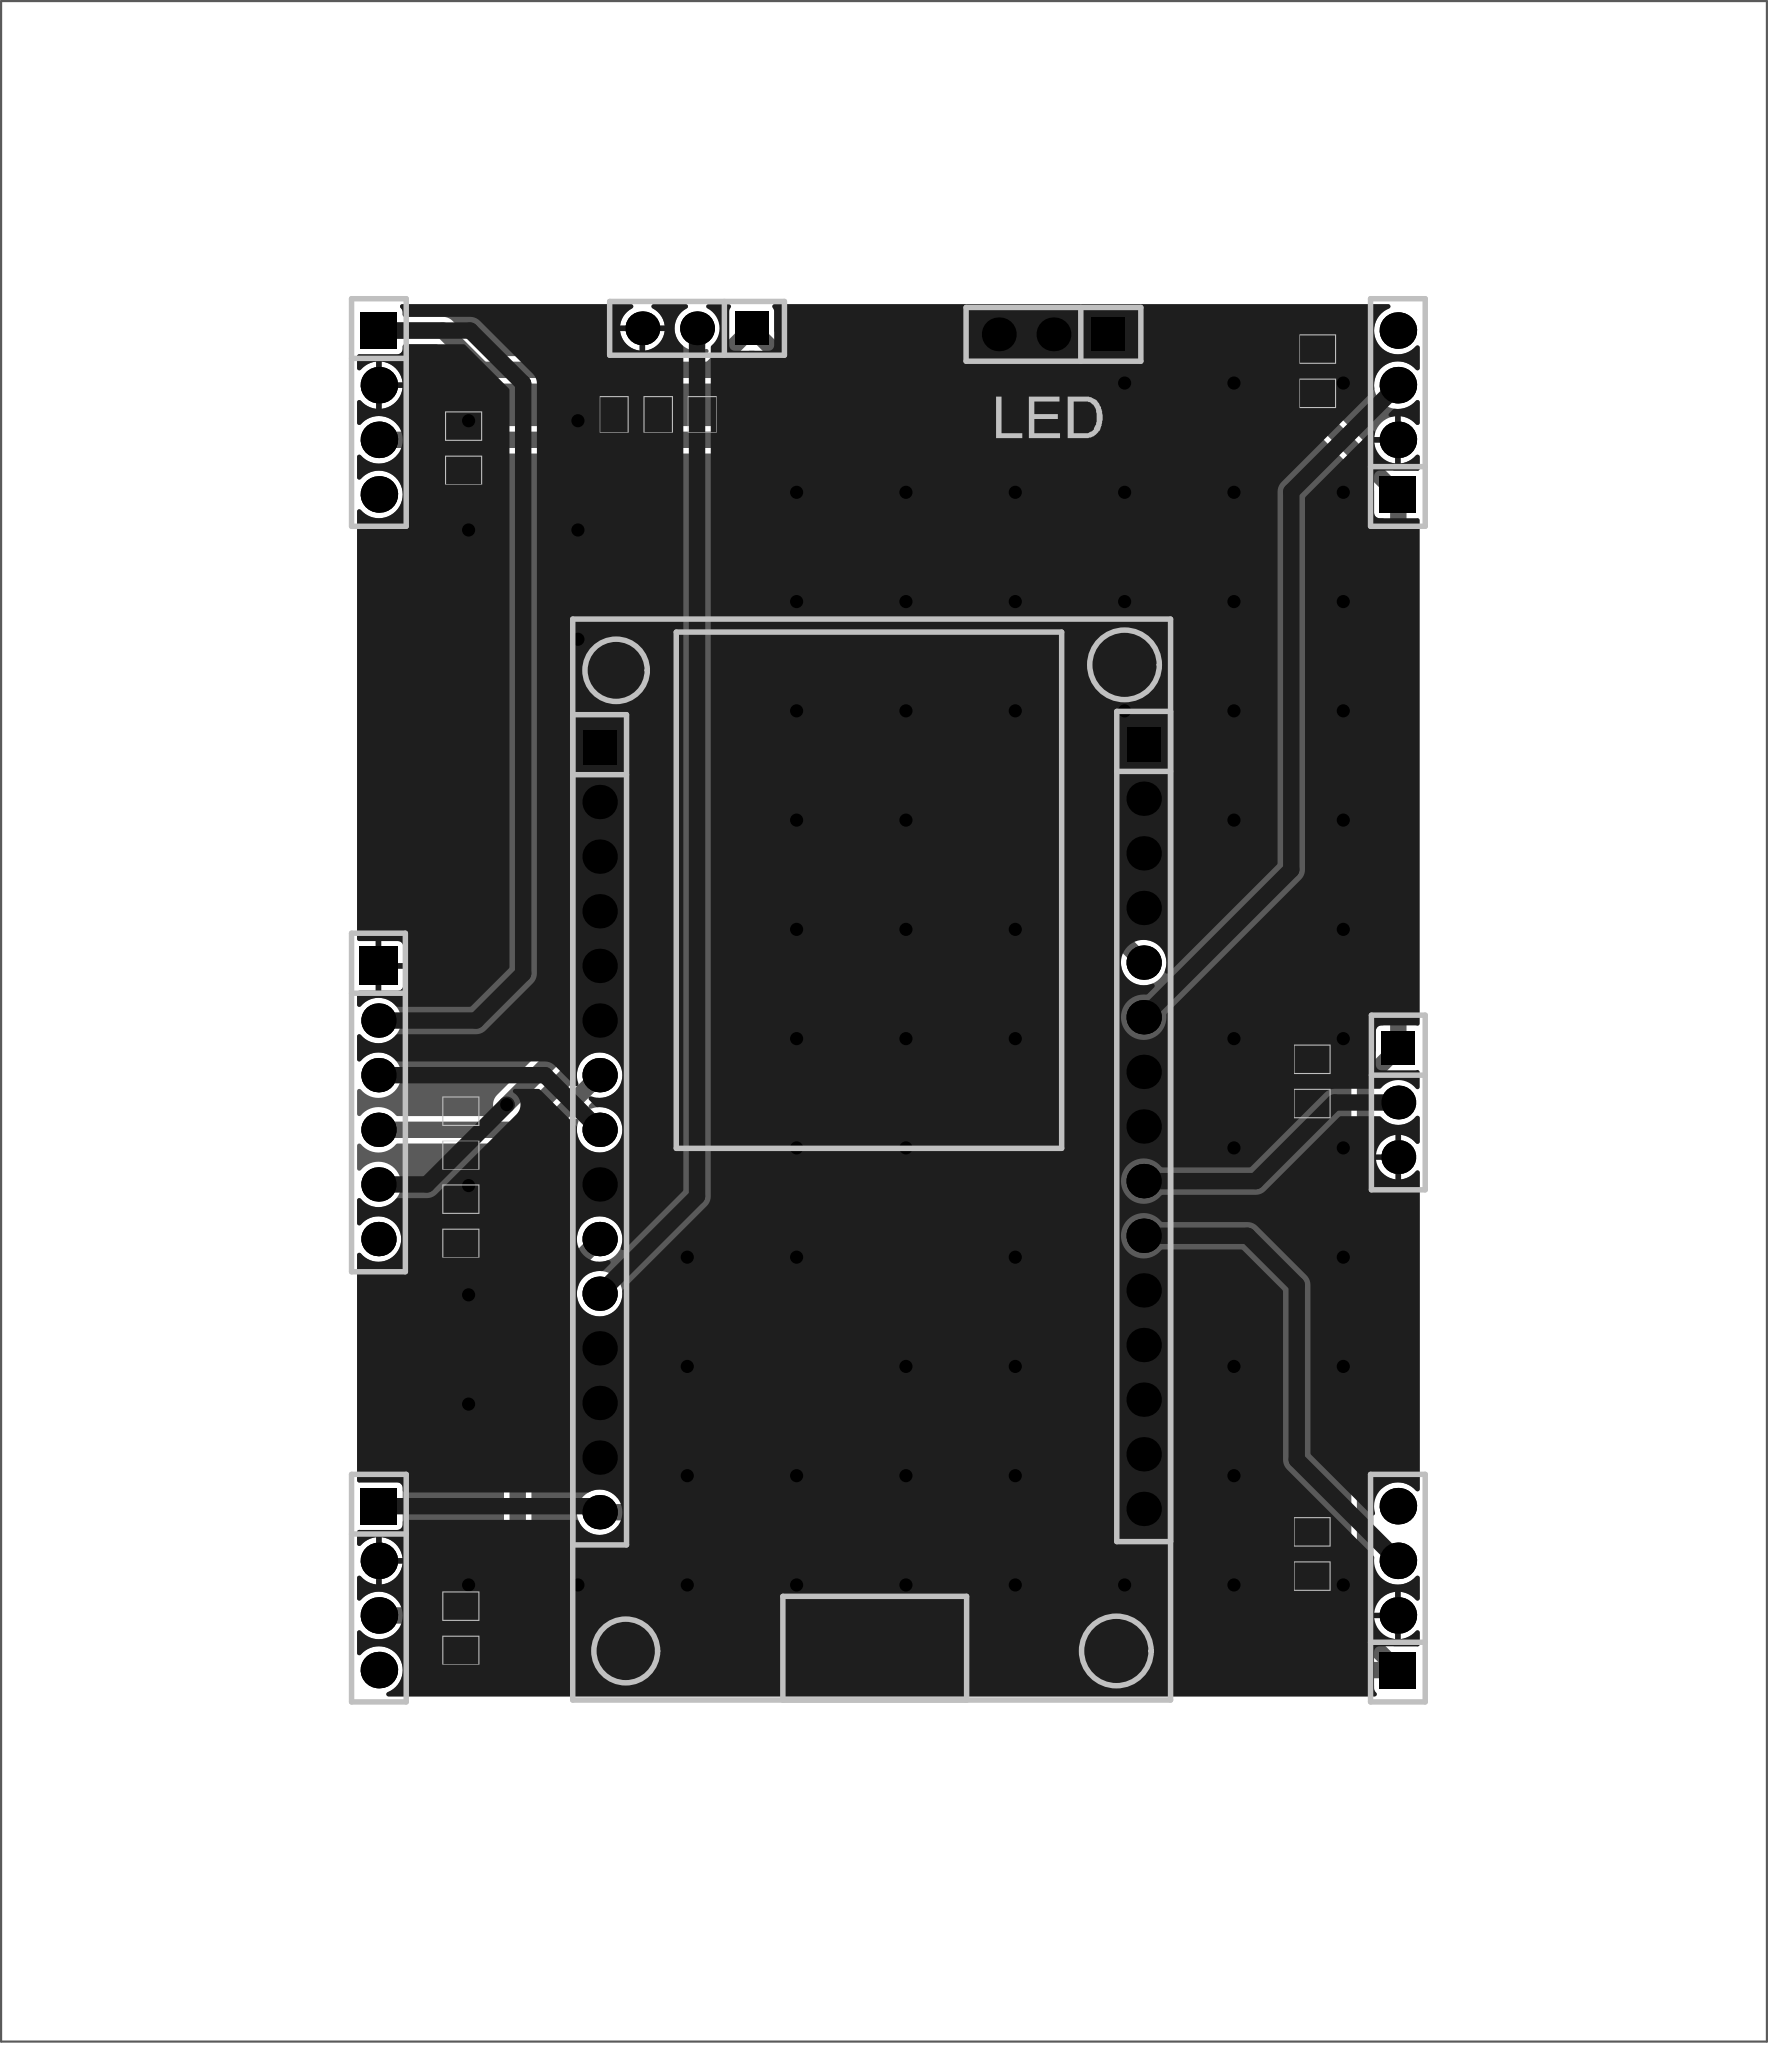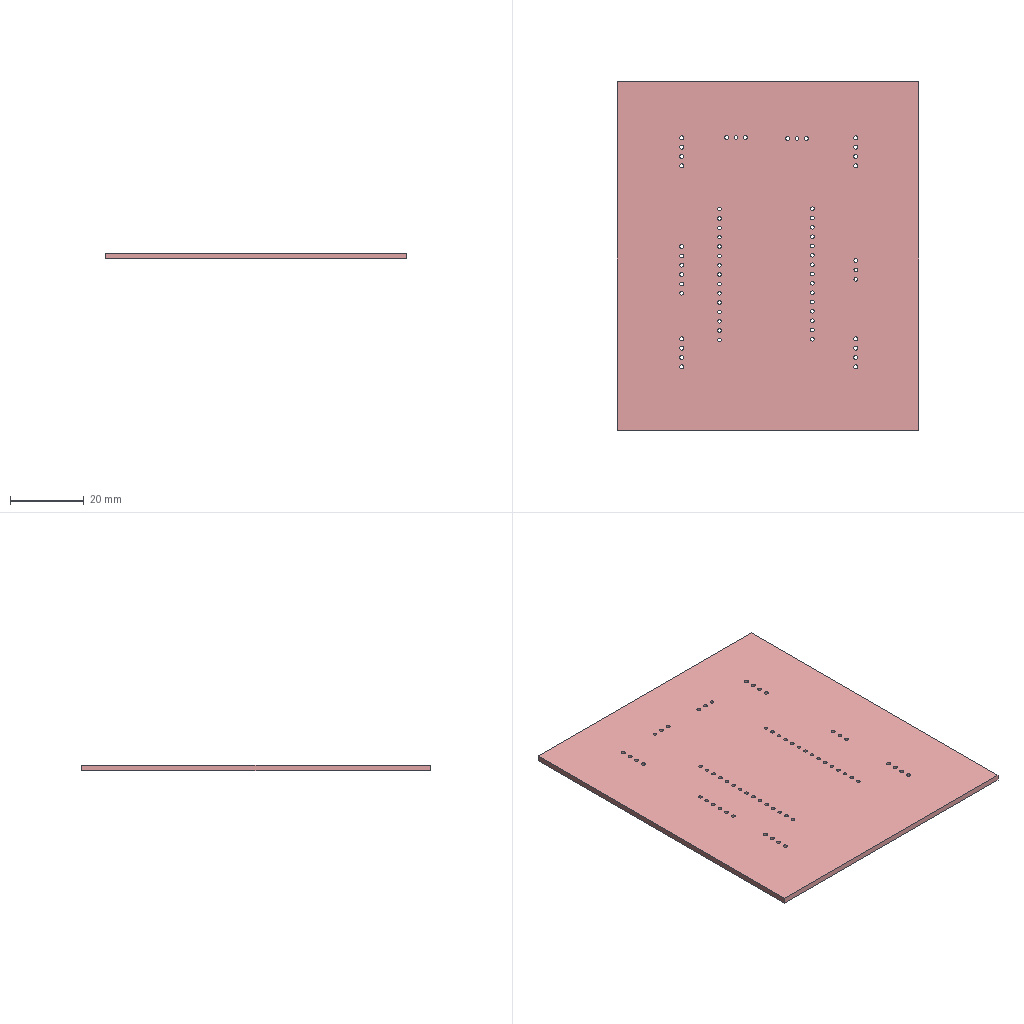Circuit board layout | Altium Designer | box 82 x 94.9 x 1.6 mm
Layer stack:
# Altium Designer layer stack of  (unit mm; dielectric type: 0 none, 1 core, 2 prepreg, 3 surface material)
index,name,kind,layer,copper_thickness_mm,dielectric_type,dielectric_thickness_mm,dielectric_material,dielectric_constant
0,Top Paste Mask Layer,other,,,,,,
1,Top Silkscreen Layer,other,,,,,,
2,Top Solder Mask Layer,dielectric,,,3,0.01,,3.3
3,Top Layer,copper,Top Layer,0.035,,,,
4,Dielectric1,dielectric,,,3,1.51,FR4,4.5
5,Bottom Layer,copper,Bottom Layer,0.035,,,,
6,Bottom Solder Mask Layer,dielectric,,,3,0.01,,3.3
7,Bottom Silkscreen Layer,other,,,,,,
8,Bottom Paste Mask Layer,other,,,,,,
# drill layer pairs: low layer,high layer
drill_pair,Top Layer,Bottom Layer
Part placement:
Designator,Comment,Layer,Footprint,Center-X(mm),Center-Y(mm),Rotation
H1,,TopLayer,HDR-TH_15P-P2.54-V-F-1,97.659,112.241,270
H2,,TopLayer,HDR-TH_15P-P2.54-V-F-1,122.936,112.395,270
H3,,TopLayer,HDR-TH_3P-P2.54-V-F,134.767,113.511,270
H4,,TopLayer,HDR-TH_6P-P2.54-V-F,87.383,113.511,270
H5,,TopLayer,HDR-TH_3P-P2.54-V-F,102.185,149.504,180
H6,,TopLayer,HDR-TH_4P-P2.54-V-F,87.403,90.932,270
H7,,TopLayer,HDR-TH_4P-P2.54-V-F,134.747,90.932,90
H8,,TopLayer,HDR-TH_4P-P2.54-V-F,134.747,145.591,90
H9,,TopLayer,HDR-TH_4P-P2.54-V-F,87.403,145.591,270
H10,,TopLayer,HDR-TH_3P-P2.54-V-F,118.745,149.225,180
Pad and via stacks:
# Altium Designer via and pad stacks of  (unit mm). Each distinct definition once, with the count of objects using it.
# via: kind,start_layer,end_layer,hole_mm,diameter_mm,mode(0 simple;1 top-mid-bottom;2 full stack),diameter_per_layer,count,example_net
# pad: kind,layer,hole_mm,hole_type(0 round;1 square;2 slot),plating,top_size,top_shape(1 round;2 rect;3 octagon;9 rounded rect),mid_size,bottom_size,mode,footprint,size_per_layer,count,example
pad,Multi-Layer,1,0,plated,1.6x1.6,1,1.6x1.6,1.6x1.6,0,HDR-TH_15P-P2.54-V-F-1,,28,H1.15
pad,Multi-Layer,1,0,plated,1.6x1.575,2,1.6x1.575,1.6x1.575,0,HDR-TH_15P-P2.54-V-F-1,,2,H1.1
pad,Multi-Layer,1.02,0,plated,1.575x1.575,1,1.575x1.575,1.575x1.575,0,HDR-TH_3P-P2.54-V-F,,6,H3.3
pad,Multi-Layer,1.02,0,plated,1.575x1.575,2,1.575x1.575,1.575x1.575,0,HDR-TH_3P-P2.54-V-F,,3,H3.1
pad,Multi-Layer,1.02,0,plated,1.6x1.6,1,1.6x1.6,1.6x1.6,0,HDR-TH_6P-P2.54-V-F,,5,H4.6
pad,Multi-Layer,1.02,0,plated,1.8x1.8,2,1.8x1.8,1.8x1.8,0,HDR-TH_6P-P2.54-V-F,,1,H4.1
pad,Multi-Layer,1.1,0,plated,1.7x1.7,2,1.7x1.7,1.7x1.7,0,HDR-TH_4P-P2.54-V-F,,4,H6.1
pad,Multi-Layer,1.1,0,plated,1.7x1.7,1,1.7x1.7,1.7x1.7,0,HDR-TH_4P-P2.54-V-F,,12,H6.2
via,Top Layer,Bottom Layer,0.3048,0.61,0,,70,GND
Copper pours:
name,layer,net,type(0 solid;1 hatched;2 none)
Top Layer-GND,Top Layer,GND,0
Bottom Layer-GND,Bottom Layer,GND,0